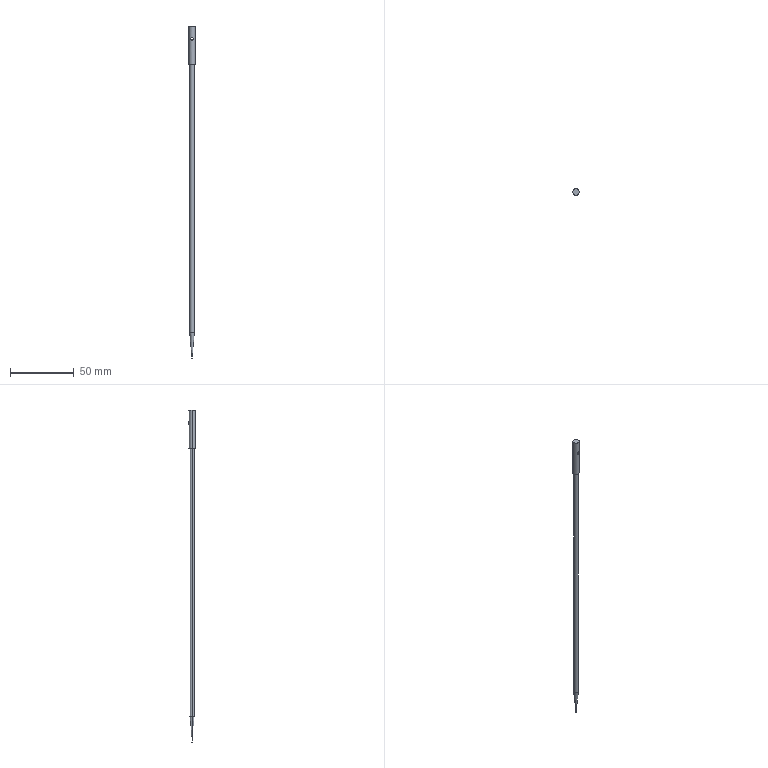Part | SolidWorks | features ICE 3, Chamfer 1, Extrusion 1 | 1 solid | 11 faces | box 5 x 5 x 260 mm | volume 2905 mm3 | cylinder 6 | plane 3 | cone 2 | commonest cylinder face diameters 2 x2 3.7 x2 5 x2
STEP:
#1=CARTESIAN_POINT('',(0.,2.5,249.));
#2=VERTEX_POINT('',#1);
#3=CARTESIAN_POINT('',(0.,2.5,251.));
#4=VERTEX_POINT('',#3);
#5=CARTESIAN_POINT('',(0.,2.5,249.));
#6=CARTESIAN_POINT('',(-0.1337,2.5,249.));
#7=CARTESIAN_POINT('',(-0.2647,2.489,249.027));
#8=CARTESIAN_POINT('',(-0.5064,2.451,249.128));
#9=CARTESIAN_POINT('',(-0.6164,2.425,249.202));
#10=CARTESIAN_POINT('',(-0.7987,2.371,249.385));
#11=CARTESIAN_POINT('',(-0.8728,2.343,249.495));
#12=CARTESIAN_POINT('',(-0.973,2.304,249.735));
#13=CARTESIAN_POINT('',(-0.9999,2.291,249.867));
#14=CARTESIAN_POINT('',(-1.,2.291,250.131));
#15=CARTESIAN_POINT('',(-0.9737,2.303,250.263));
#16=CARTESIAN_POINT('',(-0.8721,2.344,250.507));
#17=CARTESIAN_POINT('',(-0.7984,2.371,250.616));
#18=CARTESIAN_POINT('',(-0.6153,2.425,250.799));
#19=CARTESIAN_POINT('',(-0.505,2.451,250.873));
#20=CARTESIAN_POINT('',(-0.2646,2.489,250.973));
#21=CARTESIAN_POINT('',(-0.1316,2.5,251.));
#22=CARTESIAN_POINT('',(0.,2.5,251.));
#23=B_SPLINE_CURVE_WITH_KNOTS('',3,(#5,#6,#7,#8,#9,#10,#11,#12,#13,#14,#15,#16,#17,#18,#19,#20,#21,#22),.UNSPECIFIED.,.F.,.F.,(4,2,2,2,2,2,2,2,4),(0.,0.000395,0.00079,0.001185,0.00158,0.001975,0.00237,0.002765,0.00316),.UNSPECIFIED.);
#24=EDGE_CURVE('',#2,#4,#23,.T.);
#25=ORIENTED_EDGE('',*,*,#24,.T.);
#26=CARTESIAN_POINT('',(0.,-2.5,251.));
#27=VERTEX_POINT('',#26);
#28=CARTESIAN_POINT('',(0.,10.,251.));
#29=DIRECTION('',(0.,-1.,0.));
#30=VECTOR('',#29,1000.);
#31=LINE('',#28,#30);
#32=EDGE_CURVE('',#4,#27,#31,.T.);
#33=ORIENTED_EDGE('',*,*,#32,.T.);
#34=CARTESIAN_POINT('',(0.,-2.5,249.));
#35=VERTEX_POINT('',#34);
#36=CARTESIAN_POINT('',(0.,-2.5,251.));
#37=CARTESIAN_POINT('',(-0.1316,-2.5,251.));
#38=CARTESIAN_POINT('',(-0.2641,-2.489,250.973));
#39=CARTESIAN_POINT('',(-0.5061,-2.451,250.872));
#40=CARTESIAN_POINT('',(-0.6154,-2.425,250.799));
#41=CARTESIAN_POINT('',(-0.7998,-2.371,250.614));
#42=CARTESIAN_POINT('',(-0.8728,-2.343,250.505));
#43=CARTESIAN_POINT('',(-0.9734,-2.303,250.264));
#44=CARTESIAN_POINT('',(-1.,-2.291,250.132));
#45=CARTESIAN_POINT('',(-1.,-2.291,249.868));
#46=CARTESIAN_POINT('',(-0.9732,-2.303,249.736));
#47=CARTESIAN_POINT('',(-0.8728,-2.343,249.495));
#48=CARTESIAN_POINT('',(-0.7991,-2.371,249.385));
#49=CARTESIAN_POINT('',(-0.6157,-2.425,249.201));
#50=CARTESIAN_POINT('',(-0.5072,-2.451,249.128));
#51=CARTESIAN_POINT('',(-0.2636,-2.489,249.026));
#52=CARTESIAN_POINT('',(-0.1336,-2.5,249.));
#53=CARTESIAN_POINT('',(0.,-2.5,249.));
#54=B_SPLINE_CURVE_WITH_KNOTS('',3,(#36,#37,#38,#39,#40,#41,#42,#43,#44,#45,#46,#47,#48,#49,#50,#51,#52,#53),.UNSPECIFIED.,.F.,.F.,(4,2,2,2,2,2,2,2,4),(0.00316,0.003555,0.003949,0.004344,0.004739,0.005134,0.005528,0.005923,0.006318),.UNSPECIFIED.);
#55=EDGE_CURVE('',#27,#35,#54,.T.);
#56=ORIENTED_EDGE('',*,*,#55,.T.);
#57=CARTESIAN_POINT('',(0.,10.,249.));
#58=DIRECTION('',(0.,-1.,0.));
#59=VECTOR('',#58,1000.);
#60=LINE('',#57,#59);
#61=EDGE_CURVE('',#2,#35,#60,.T.);
#62=ORIENTED_EDGE('',*,*,#61,.F.);
#63=EDGE_LOOP('',(#25,#33,#56,#62));
#64=FACE_OUTER_BOUND('',#63,.T.);
#65=CARTESIAN_POINT('',(0.,10.,250.));
#66=DIRECTION('',(0.,-1.,0.));
#67=DIRECTION('',(0.,0.,-1.));
#68=AXIS2_PLACEMENT_3D('',#65,#66,#67);
#69=CYLINDRICAL_SURFACE('',#68,1.);
#70=ADVANCED_FACE('',(#64),#69,.F.);
#71=CARTESIAN_POINT('',(-0.05,0.,0.));
#72=VERTEX_POINT('',#71);
#73=CARTESIAN_POINT('',(0.05,0.,0.));
#74=VERTEX_POINT('',#73);
#75=CARTESIAN_POINT('',(0.,0.,0.));
#76=DIRECTION('',(0.,0.,-1.));
#77=DIRECTION('',(1.,0.,0.));
#78=AXIS2_PLACEMENT_3D('',#75,#76,#77);
#79=CIRCLE('',#78,0.05);
#80=EDGE_CURVE('',#72,#74,#79,.T.);
#81=ORIENTED_EDGE('',*,*,#80,.F.);
#82=CARTESIAN_POINT('',(-1.85,0.,20.));
#83=VERTEX_POINT('',#82);
#84=CARTESIAN_POINT('',(-1.85,0.,20.));
#85=DIRECTION('',(-0.08964,0.,0.996));
#86=VECTOR('',#85,1000.);
#87=LINE('',#84,#86);
#88=EDGE_CURVE('',#72,#83,#87,.T.);
#89=ORIENTED_EDGE('',*,*,#88,.T.);
#90=CARTESIAN_POINT('',(1.85,0.,20.));
#91=VERTEX_POINT('',#90);
#92=CARTESIAN_POINT('',(0.,0.,20.));
#93=DIRECTION('',(0.,0.,1.));
#94=DIRECTION('',(1.,0.,0.));
#95=AXIS2_PLACEMENT_3D('',#92,#93,#94);
#96=CIRCLE('',#95,1.85);
#97=EDGE_CURVE('',#91,#83,#96,.T.);
#98=ORIENTED_EDGE('',*,*,#97,.F.);
#99=CARTESIAN_POINT('',(1.85,0.,20.));
#100=DIRECTION('',(0.08964,0.,0.996));
#101=VECTOR('',#100,1000.);
#102=LINE('',#99,#101);
#103=EDGE_CURVE('',#74,#91,#102,.T.);
#104=ORIENTED_EDGE('',*,*,#103,.F.);
#105=EDGE_LOOP('',(#81,#89,#98,#104));
#106=FACE_OUTER_BOUND('',#105,.T.);
#107=CARTESIAN_POINT('',(0.,0.,20.));
#108=DIRECTION('',(0.,0.,1.));
#109=DIRECTION('',(1.,0.,0.));
#110=AXIS2_PLACEMENT_3D('',#107,#108,#109);
#111=CONICAL_SURFACE('',#110,1.85,0.08976);
#112=ADVANCED_FACE('',(#106),#111,.T.);
#113=CARTESIAN_POINT('',(1.85,0.,230.));
#114=VERTEX_POINT('',#113);
#115=CARTESIAN_POINT('',(-1.85,0.,230.));
#116=VERTEX_POINT('',#115);
#117=CARTESIAN_POINT('',(0.,0.,230.));
#118=DIRECTION('',(0.,0.,1.));
#119=DIRECTION('',(1.,0.,0.));
#120=AXIS2_PLACEMENT_3D('',#117,#118,#119);
#121=CIRCLE('',#120,1.85);
#122=EDGE_CURVE('',#114,#116,#121,.T.);
#123=ORIENTED_EDGE('',*,*,#122,.F.);
#124=CARTESIAN_POINT('',(1.85,0.,230.));
#125=DIRECTION('',(0.,0.,-1.));
#126=VECTOR('',#125,1000.);
#127=LINE('',#124,#126);
#128=EDGE_CURVE('',#114,#91,#127,.T.);
#129=ORIENTED_EDGE('',*,*,#128,.T.);
#130=ORIENTED_EDGE('',*,*,#97,.T.);
#131=CARTESIAN_POINT('',(-1.85,0.,230.));
#132=DIRECTION('',(0.,0.,-1.));
#133=VECTOR('',#132,1000.);
#134=LINE('',#131,#133);
#135=EDGE_CURVE('',#116,#83,#134,.T.);
#136=ORIENTED_EDGE('',*,*,#135,.F.);
#137=EDGE_LOOP('',(#123,#129,#130,#136));
#138=FACE_OUTER_BOUND('',#137,.T.);
#139=CARTESIAN_POINT('',(0.,0.,230.));
#140=DIRECTION('',(0.,0.,-1.));
#141=DIRECTION('',(-1.,0.,0.));
#142=AXIS2_PLACEMENT_3D('',#139,#140,#141);
#143=CYLINDRICAL_SURFACE('',#142,1.85);
#144=ADVANCED_FACE('',(#138),#143,.T.);
#145=ORIENTED_EDGE('',*,*,#24,.F.);
#146=CARTESIAN_POINT('',(0.,2.5,251.));
#147=CARTESIAN_POINT('',(0.1316,2.5,251.));
#148=CARTESIAN_POINT('',(0.2641,2.489,250.973));
#149=CARTESIAN_POINT('',(0.5061,2.451,250.872));
#150=CARTESIAN_POINT('',(0.6154,2.425,250.799));
#151=CARTESIAN_POINT('',(0.7998,2.371,250.614));
#152=CARTESIAN_POINT('',(0.8728,2.343,250.505));
#153=CARTESIAN_POINT('',(0.9734,2.303,250.264));
#154=CARTESIAN_POINT('',(1.,2.291,250.132));
#155=CARTESIAN_POINT('',(1.,2.291,249.868));
#156=CARTESIAN_POINT('',(0.9732,2.303,249.736));
#157=CARTESIAN_POINT('',(0.8728,2.343,249.495));
#158=CARTESIAN_POINT('',(0.7991,2.371,249.385));
#159=CARTESIAN_POINT('',(0.6157,2.425,249.201));
#160=CARTESIAN_POINT('',(0.5072,2.451,249.128));
#161=CARTESIAN_POINT('',(0.2636,2.489,249.026));
#162=CARTESIAN_POINT('',(0.1336,2.5,249.));
#163=CARTESIAN_POINT('',(0.,2.5,249.));
#164=B_SPLINE_CURVE_WITH_KNOTS('',3,(#146,#147,#148,#149,#150,#151,#152,#153,#154,#155,#156,#157,#158,#159,#160,#161,#162,#163),.UNSPECIFIED.,.F.,.F.,(4,2,2,2,2,2,2,2,4),(0.00316,0.003555,0.003949,0.004344,0.004739,0.005134,0.005528,0.005923,0.006318),.UNSPECIFIED.);
#165=EDGE_CURVE('',#4,#2,#164,.T.);
#166=ORIENTED_EDGE('',*,*,#165,.F.);
#167=EDGE_LOOP('',(#145,#166));
#168=FACE_BOUND('',#167,.T.);
#169=CARTESIAN_POINT('',(2.5,0.,260.));
#170=VERTEX_POINT('',#169);
#171=CARTESIAN_POINT('',(-2.5,0.,260.));
#172=VERTEX_POINT('',#171);
#173=CARTESIAN_POINT('',(0.,0.,260.));
#174=DIRECTION('',(0.,0.,1.));
#175=DIRECTION('',(1.,0.,0.));
#176=AXIS2_PLACEMENT_3D('',#173,#174,#175);
#177=CIRCLE('',#176,2.5);
#178=EDGE_CURVE('',#170,#172,#177,.T.);
#179=ORIENTED_EDGE('',*,*,#178,.F.);
#180=CARTESIAN_POINT('',(2.5,0.,230.));
#181=VERTEX_POINT('',#180);
#182=CARTESIAN_POINT('',(2.5,0.,260.));
#183=DIRECTION('',(0.,0.,-1.));
#184=VECTOR('',#183,1000.);
#185=LINE('',#182,#184);
#186=EDGE_CURVE('',#170,#181,#185,.T.);
#187=ORIENTED_EDGE('',*,*,#186,.T.);
#188=CARTESIAN_POINT('',(-2.5,0.,230.));
#189=VERTEX_POINT('',#188);
#190=CARTESIAN_POINT('',(0.,0.,230.));
#191=DIRECTION('',(0.,0.,1.));
#192=DIRECTION('',(1.,0.,0.));
#193=AXIS2_PLACEMENT_3D('',#190,#191,#192);
#194=CIRCLE('',#193,2.5);
#195=EDGE_CURVE('',#181,#189,#194,.T.);
#196=ORIENTED_EDGE('',*,*,#195,.T.);
#197=CARTESIAN_POINT('',(-2.5,0.,260.));
#198=DIRECTION('',(0.,0.,-1.));
#199=VECTOR('',#198,1000.);
#200=LINE('',#197,#199);
#201=EDGE_CURVE('',#172,#189,#200,.T.);
#202=ORIENTED_EDGE('',*,*,#201,.F.);
#203=EDGE_LOOP('',(#179,#187,#196,#202));
#204=FACE_OUTER_BOUND('',#203,.T.);
#205=CARTESIAN_POINT('',(0.,0.,260.));
#206=DIRECTION('',(0.,0.,-1.));
#207=DIRECTION('',(-1.,0.,0.));
#208=AXIS2_PLACEMENT_3D('',#205,#206,#207);
#209=CYLINDRICAL_SURFACE('',#208,2.5);
#210=ADVANCED_FACE('',(#168,#204),#209,.T.);
#211=ORIENTED_EDGE('',*,*,#186,.F.);
#212=CARTESIAN_POINT('',(0.,0.,260.));
#213=DIRECTION('',(0.,0.,1.));
#214=DIRECTION('',(1.,0.,0.));
#215=AXIS2_PLACEMENT_3D('',#212,#213,#214);
#216=CIRCLE('',#215,2.5);
#217=EDGE_CURVE('',#172,#170,#216,.T.);
#218=ORIENTED_EDGE('',*,*,#217,.F.);
#219=ORIENTED_EDGE('',*,*,#201,.T.);
#220=CARTESIAN_POINT('',(0.,0.,230.));
#221=DIRECTION('',(0.,0.,1.));
#222=DIRECTION('',(1.,0.,0.));
#223=AXIS2_PLACEMENT_3D('',#220,#221,#222);
#224=CIRCLE('',#223,2.5);
#225=EDGE_CURVE('',#189,#181,#224,.T.);
#226=ORIENTED_EDGE('',*,*,#225,.T.);
#227=EDGE_LOOP('',(#211,#218,#219,#226));
#228=FACE_OUTER_BOUND('',#227,.T.);
#229=CARTESIAN_POINT('',(0.,-2.5,249.));
#230=CARTESIAN_POINT('',(0.1337,-2.5,249.));
#231=CARTESIAN_POINT('',(0.2647,-2.489,249.027));
#232=CARTESIAN_POINT('',(0.5064,-2.451,249.128));
#233=CARTESIAN_POINT('',(0.6164,-2.425,249.202));
#234=CARTESIAN_POINT('',(0.7987,-2.371,249.385));
#235=CARTESIAN_POINT('',(0.8728,-2.343,249.495));
#236=CARTESIAN_POINT('',(0.973,-2.304,249.735));
#237=CARTESIAN_POINT('',(0.9999,-2.291,249.867));
#238=CARTESIAN_POINT('',(1.,-2.291,250.131));
#239=CARTESIAN_POINT('',(0.9737,-2.303,250.263));
#240=CARTESIAN_POINT('',(0.8721,-2.344,250.507));
#241=CARTESIAN_POINT('',(0.7984,-2.371,250.616));
#242=CARTESIAN_POINT('',(0.6153,-2.425,250.799));
#243=CARTESIAN_POINT('',(0.505,-2.451,250.873));
#244=CARTESIAN_POINT('',(0.2646,-2.489,250.973));
#245=CARTESIAN_POINT('',(0.1316,-2.5,251.));
#246=CARTESIAN_POINT('',(0.,-2.5,251.));
#247=B_SPLINE_CURVE_WITH_KNOTS('',3,(#229,#230,#231,#232,#233,#234,#235,#236,#237,#238,#239,#240,#241,#242,#243,#244,#245,#246),.UNSPECIFIED.,.F.,.F.,(4,2,2,2,2,2,2,2,4),(0.,0.000395,0.00079,0.001185,0.00158,0.001975,0.00237,0.002765,0.00316),.UNSPECIFIED.);
#248=EDGE_CURVE('',#35,#27,#247,.T.);
#249=ORIENTED_EDGE('',*,*,#248,.F.);
#250=ORIENTED_EDGE('',*,*,#55,.F.);
#251=EDGE_LOOP('',(#249,#250));
#252=FACE_BOUND('',#251,.T.);
#253=CARTESIAN_POINT('',(0.,0.,260.));
#254=DIRECTION('',(0.,0.,-1.));
#255=DIRECTION('',(-1.,0.,0.));
#256=AXIS2_PLACEMENT_3D('',#253,#254,#255);
#257=CYLINDRICAL_SURFACE('',#256,2.5);
#258=ADVANCED_FACE('',(#228,#252),#257,.T.);
#259=ORIENTED_EDGE('',*,*,#128,.F.);
#260=CARTESIAN_POINT('',(0.,0.,230.));
#261=DIRECTION('',(0.,0.,1.));
#262=DIRECTION('',(1.,0.,0.));
#263=AXIS2_PLACEMENT_3D('',#260,#261,#262);
#264=CIRCLE('',#263,1.85);
#265=EDGE_CURVE('',#116,#114,#264,.T.);
#266=ORIENTED_EDGE('',*,*,#265,.F.);
#267=ORIENTED_EDGE('',*,*,#135,.T.);
#268=CARTESIAN_POINT('',(0.,0.,20.));
#269=DIRECTION('',(0.,0.,1.));
#270=DIRECTION('',(1.,0.,0.));
#271=AXIS2_PLACEMENT_3D('',#268,#269,#270);
#272=CIRCLE('',#271,1.85);
#273=EDGE_CURVE('',#83,#91,#272,.T.);
#274=ORIENTED_EDGE('',*,*,#273,.T.);
#275=EDGE_LOOP('',(#259,#266,#267,#274));
#276=FACE_OUTER_BOUND('',#275,.T.);
#277=CARTESIAN_POINT('',(0.,0.,230.));
#278=DIRECTION('',(0.,0.,-1.));
#279=DIRECTION('',(-1.,0.,0.));
#280=AXIS2_PLACEMENT_3D('',#277,#278,#279);
#281=CYLINDRICAL_SURFACE('',#280,1.85);
#282=ADVANCED_FACE('',(#276),#281,.T.);
#283=CARTESIAN_POINT('',(0.,0.,0.));
#284=DIRECTION('',(0.,0.,-1.));
#285=DIRECTION('',(1.,0.,0.));
#286=AXIS2_PLACEMENT_3D('',#283,#284,#285);
#287=CIRCLE('',#286,0.05);
#288=EDGE_CURVE('',#74,#72,#287,.T.);
#289=ORIENTED_EDGE('',*,*,#288,.T.);
#290=ORIENTED_EDGE('',*,*,#80,.T.);
#291=EDGE_LOOP('',(#289,#290));
#292=FACE_OUTER_BOUND('',#291,.T.);
#293=CARTESIAN_POINT('',(0.,0.,0.));
#294=DIRECTION('',(0.,0.,1.));
#295=DIRECTION('',(1.,0.,0.));
#296=AXIS2_PLACEMENT_3D('',#293,#294,#295);
#297=PLANE('',#296);
#298=ADVANCED_FACE('',(#292),#297,.F.);
#299=ORIENTED_EDGE('',*,*,#225,.F.);
#300=ORIENTED_EDGE('',*,*,#195,.F.);
#301=EDGE_LOOP('',(#299,#300));
#302=FACE_OUTER_BOUND('',#301,.T.);
#303=ORIENTED_EDGE('',*,*,#265,.T.);
#304=ORIENTED_EDGE('',*,*,#122,.T.);
#305=EDGE_LOOP('',(#303,#304));
#306=FACE_BOUND('',#305,.T.);
#307=CARTESIAN_POINT('',(0.,0.,230.));
#308=DIRECTION('',(0.,0.,1.));
#309=DIRECTION('',(1.,0.,0.));
#310=AXIS2_PLACEMENT_3D('',#307,#308,#309);
#311=PLANE('',#310);
#312=ADVANCED_FACE('',(#302,#306),#311,.F.);
#313=ORIENTED_EDGE('',*,*,#217,.T.);
#314=ORIENTED_EDGE('',*,*,#178,.T.);
#315=EDGE_LOOP('',(#313,#314));
#316=FACE_OUTER_BOUND('',#315,.T.);
#317=CARTESIAN_POINT('',(0.,0.,260.));
#318=DIRECTION('',(0.,0.,1.));
#319=DIRECTION('',(1.,0.,0.));
#320=AXIS2_PLACEMENT_3D('',#317,#318,#319);
#321=PLANE('',#320);
#322=ADVANCED_FACE('',(#316),#321,.T.);
#323=ORIENTED_EDGE('',*,*,#88,.F.);
#324=ORIENTED_EDGE('',*,*,#288,.F.);
#325=ORIENTED_EDGE('',*,*,#103,.T.);
#326=ORIENTED_EDGE('',*,*,#273,.F.);
#327=EDGE_LOOP('',(#323,#324,#325,#326));
#328=FACE_OUTER_BOUND('',#327,.T.);
#329=CARTESIAN_POINT('',(0.,0.,20.));
#330=DIRECTION('',(0.,0.,1.));
#331=DIRECTION('',(1.,0.,0.));
#332=AXIS2_PLACEMENT_3D('',#329,#330,#331);
#333=CONICAL_SURFACE('',#332,1.85,0.08976);
#334=ADVANCED_FACE('',(#328),#333,.T.);
#335=ORIENTED_EDGE('',*,*,#32,.F.);
#336=ORIENTED_EDGE('',*,*,#165,.T.);
#337=ORIENTED_EDGE('',*,*,#61,.T.);
#338=ORIENTED_EDGE('',*,*,#248,.T.);
#339=EDGE_LOOP('',(#335,#336,#337,#338));
#340=FACE_OUTER_BOUND('',#339,.T.);
#341=CARTESIAN_POINT('',(0.,10.,250.));
#342=DIRECTION('',(0.,-1.,0.));
#343=DIRECTION('',(0.,0.,-1.));
#344=AXIS2_PLACEMENT_3D('',#341,#342,#343);
#345=CYLINDRICAL_SURFACE('',#344,1.);
#346=ADVANCED_FACE('',(#340),#345,.F.);
#347=CLOSED_SHELL('',(#70,#112,#144,#210,#258,#282,#298,#312,#322,#334,#346));
#348=MANIFOLD_SOLID_BREP('',#347);
#349=CARTESIAN_POINT('',(0.,0.,0.));
#350=DIRECTION('',(0.,0.,1.));
#351=DIRECTION('',(1.,0.,0.));
#352=AXIS2_PLACEMENT_3D('',#349,#350,#351);
#353=(LENGTH_UNIT()NAMED_UNIT(*)SI_UNIT(.MILLI.,.METRE.));
#354=UNCERTAINTY_MEASURE_WITH_UNIT(LENGTH_MEASURE(0.00001),#353,'','');
#355=(NAMED_UNIT(*)PLANE_ANGLE_UNIT()SI_UNIT($,.RADIAN.));
#356=(NAMED_UNIT(*)SI_UNIT($,.STERADIAN.)SOLID_ANGLE_UNIT());
#357=(GEOMETRIC_REPRESENTATION_CONTEXT(3)GLOBAL_UNCERTAINTY_ASSIGNED_CONTEXT((#354))GLOBAL_UNIT_ASSIGNED_CONTEXT((#353,#355,#356))REPRESENTATION_CONTEXT('',''));
#358=ADVANCED_BREP_SHAPE_REPRESENTATION('',(#348,#352),#357);